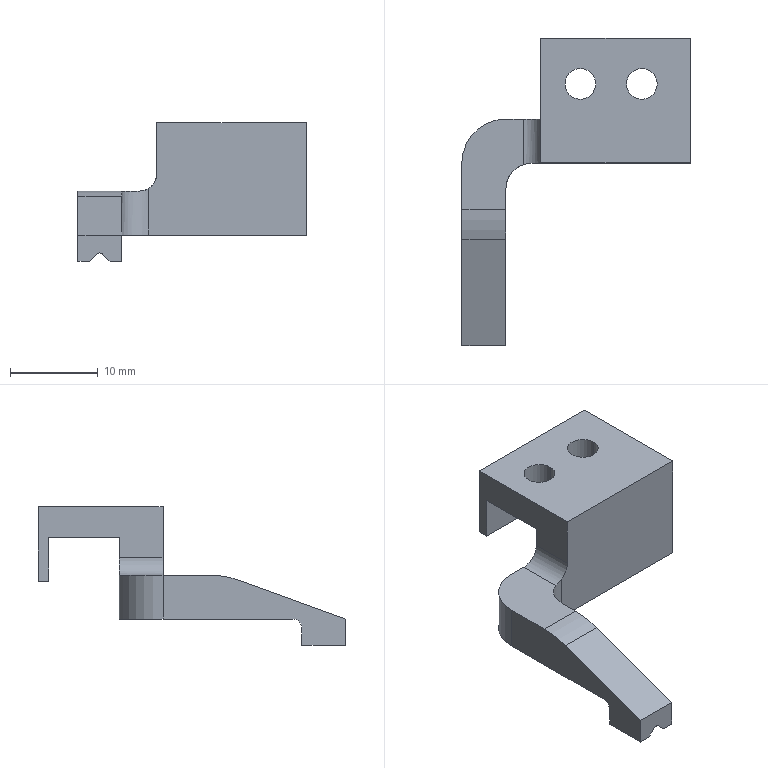Part | SolidWorks | features ICE 10, Fillet 6, Chamfer 1, Extrusion 1, HoleWzd 1, MoveFace 1 | 1 solid | 31 faces | box 26 x 35 x 15.8 mm | volume 2299 mm3 | plane 20 | cylinder 11 | commonest cylinder face diameters 3.5 x4 1 x2 2 x1 4 x1 6 x1 10 x1
STEP:
#1=CARTESIAN_POINT('',(-10.5,-18.5,-6.943));
#2=VERTEX_POINT('',#1);
#3=CARTESIAN_POINT('',(-10.146,-18.5,-7.089));
#4=VERTEX_POINT('',#3);
#5=CARTESIAN_POINT('',(-10.5,-18.5,-7.443));
#6=DIRECTION('',(0.,1.,0.));
#7=DIRECTION('',(0.,0.,1.));
#8=AXIS2_PLACEMENT_3D('',#5,#6,#7);
#9=CIRCLE('',#8,0.5);
#10=EDGE_CURVE('',#2,#4,#9,.T.);
#11=ORIENTED_EDGE('',*,*,#10,.F.);
#12=CARTESIAN_POINT('',(-10.5,-13.5,-6.943));
#13=VERTEX_POINT('',#12);
#14=CARTESIAN_POINT('',(-10.5,4.5,-6.943));
#15=DIRECTION('',(0.,1.,0.));
#16=VECTOR('',#15,1000.);
#17=LINE('',#14,#16);
#18=EDGE_CURVE('',#2,#13,#17,.T.);
#19=ORIENTED_EDGE('',*,*,#18,.T.);
#20=CARTESIAN_POINT('',(-10.146,-13.5,-7.089));
#21=VERTEX_POINT('',#20);
#22=CARTESIAN_POINT('',(-10.5,-13.5,-7.443));
#23=DIRECTION('',(0.,-1.,0.));
#24=DIRECTION('',(0.,0.,1.));
#25=AXIS2_PLACEMENT_3D('',#22,#23,#24);
#26=CIRCLE('',#25,0.5);
#27=EDGE_CURVE('',#21,#13,#26,.T.);
#28=ORIENTED_EDGE('',*,*,#27,.F.);
#29=CARTESIAN_POINT('',(-10.146,-11.5,-7.089));
#30=DIRECTION('',(0.,1.,0.));
#31=VECTOR('',#30,1000.);
#32=LINE('',#29,#31);
#33=EDGE_CURVE('',#4,#21,#32,.T.);
#34=ORIENTED_EDGE('',*,*,#33,.F.);
#35=EDGE_LOOP('',(#11,#19,#28,#34));
#36=FACE_OUTER_BOUND('',#35,.T.);
#37=CARTESIAN_POINT('',(-10.5,4.5,-7.443));
#38=DIRECTION('',(0.,1.,0.));
#39=DIRECTION('',(0.,0.,1.));
#40=AXIS2_PLACEMENT_3D('',#37,#38,#39);
#41=CYLINDRICAL_SURFACE('',#40,0.5);
#42=ADVANCED_FACE('',(#36),#41,.F.);
#43=CARTESIAN_POINT('',(2.25,11.3,4.4));
#44=VERTEX_POINT('',#43);
#45=CARTESIAN_POINT('',(-1.25,11.3,4.4));
#46=VERTEX_POINT('',#45);
#47=CARTESIAN_POINT('',(0.5,11.3,4.4));
#48=DIRECTION('',(0.,0.,-1.));
#49=DIRECTION('',(1.,0.,0.));
#50=AXIS2_PLACEMENT_3D('',#47,#48,#49);
#51=CIRCLE('',#50,1.75);
#52=EDGE_CURVE('',#44,#46,#51,.T.);
#53=ORIENTED_EDGE('',*,*,#52,.T.);
#54=CARTESIAN_POINT('',(-1.25,11.3,7.9));
#55=VERTEX_POINT('',#54);
#56=CARTESIAN_POINT('',(-1.25,11.3,7.9));
#57=DIRECTION('',(0.,0.,1.));
#58=VECTOR('',#57,1000.);
#59=LINE('',#56,#58);
#60=EDGE_CURVE('',#46,#55,#59,.T.);
#61=ORIENTED_EDGE('',*,*,#60,.T.);
#62=CARTESIAN_POINT('',(2.25,11.3,7.9));
#63=VERTEX_POINT('',#62);
#64=CARTESIAN_POINT('',(0.5,11.3,7.9));
#65=DIRECTION('',(0.,0.,1.));
#66=DIRECTION('',(1.,0.,0.));
#67=AXIS2_PLACEMENT_3D('',#64,#65,#66);
#68=CIRCLE('',#67,1.75);
#69=EDGE_CURVE('',#55,#63,#68,.T.);
#70=ORIENTED_EDGE('',*,*,#69,.T.);
#71=CARTESIAN_POINT('',(2.25,11.3,7.9));
#72=DIRECTION('',(0.,0.,1.));
#73=VECTOR('',#72,1000.);
#74=LINE('',#71,#73);
#75=EDGE_CURVE('',#44,#63,#74,.T.);
#76=ORIENTED_EDGE('',*,*,#75,.F.);
#77=EDGE_LOOP('',(#53,#61,#70,#76));
#78=FACE_OUTER_BOUND('',#77,.T.);
#79=CARTESIAN_POINT('',(0.5,11.3,7.9));
#80=DIRECTION('',(0.,0.,1.));
#81=DIRECTION('',(1.,0.,0.));
#82=AXIS2_PLACEMENT_3D('',#79,#80,#81);
#83=CYLINDRICAL_SURFACE('',#82,1.75);
#84=ADVANCED_FACE('',(#78),#83,.F.);
#85=CARTESIAN_POINT('',(9.25,11.3,4.4));
#86=VERTEX_POINT('',#85);
#87=CARTESIAN_POINT('',(5.75,11.3,4.4));
#88=VERTEX_POINT('',#87);
#89=CARTESIAN_POINT('',(7.5,11.3,4.4));
#90=DIRECTION('',(0.,0.,-1.));
#91=DIRECTION('',(1.,0.,0.));
#92=AXIS2_PLACEMENT_3D('',#89,#90,#91);
#93=CIRCLE('',#92,1.75);
#94=EDGE_CURVE('',#86,#88,#93,.T.);
#95=ORIENTED_EDGE('',*,*,#94,.T.);
#96=CARTESIAN_POINT('',(5.75,11.3,7.9));
#97=VERTEX_POINT('',#96);
#98=CARTESIAN_POINT('',(5.75,11.3,7.9));
#99=DIRECTION('',(0.,0.,1.));
#100=VECTOR('',#99,1000.);
#101=LINE('',#98,#100);
#102=EDGE_CURVE('',#88,#97,#101,.T.);
#103=ORIENTED_EDGE('',*,*,#102,.T.);
#104=CARTESIAN_POINT('',(9.25,11.3,7.9));
#105=VERTEX_POINT('',#104);
#106=CARTESIAN_POINT('',(7.5,11.3,7.9));
#107=DIRECTION('',(0.,0.,1.));
#108=DIRECTION('',(1.,0.,0.));
#109=AXIS2_PLACEMENT_3D('',#106,#107,#108);
#110=CIRCLE('',#109,1.75);
#111=EDGE_CURVE('',#97,#105,#110,.T.);
#112=ORIENTED_EDGE('',*,*,#111,.T.);
#113=CARTESIAN_POINT('',(9.25,11.3,7.9));
#114=DIRECTION('',(0.,0.,1.));
#115=VECTOR('',#114,1000.);
#116=LINE('',#113,#115);
#117=EDGE_CURVE('',#86,#105,#116,.T.);
#118=ORIENTED_EDGE('',*,*,#117,.F.);
#119=EDGE_LOOP('',(#95,#103,#112,#118));
#120=FACE_OUTER_BOUND('',#119,.T.);
#121=CARTESIAN_POINT('',(7.5,11.3,7.9));
#122=DIRECTION('',(0.,0.,1.));
#123=DIRECTION('',(1.,0.,0.));
#124=AXIS2_PLACEMENT_3D('',#121,#122,#123);
#125=CYLINDRICAL_SURFACE('',#124,1.75);
#126=ADVANCED_FACE('',(#120),#125,.F.);
#127=CARTESIAN_POINT('',(-9.336,-18.5,-7.9));
#128=VERTEX_POINT('',#127);
#129=CARTESIAN_POINT('',(-8.,-18.5,-7.9));
#130=VERTEX_POINT('',#129);
#131=CARTESIAN_POINT('',(-13.,-18.5,-7.9));
#132=DIRECTION('',(1.,0.,0.));
#133=VECTOR('',#132,1000.);
#134=LINE('',#131,#133);
#135=EDGE_CURVE('',#128,#130,#134,.T.);
#136=ORIENTED_EDGE('',*,*,#135,.F.);
#137=CARTESIAN_POINT('',(-9.336,-13.5,-7.9));
#138=VERTEX_POINT('',#137);
#139=CARTESIAN_POINT('',(-9.336,0.,-7.9));
#140=DIRECTION('',(0.,1.,0.));
#141=VECTOR('',#140,1000.);
#142=LINE('',#139,#141);
#143=EDGE_CURVE('',#128,#138,#142,.T.);
#144=ORIENTED_EDGE('',*,*,#143,.T.);
#145=CARTESIAN_POINT('',(-8.,-13.5,-7.9));
#146=VERTEX_POINT('',#145);
#147=CARTESIAN_POINT('',(-13.,-13.5,-7.9));
#148=DIRECTION('',(1.,0.,0.));
#149=VECTOR('',#148,1000.);
#150=LINE('',#147,#149);
#151=EDGE_CURVE('',#138,#146,#150,.T.);
#152=ORIENTED_EDGE('',*,*,#151,.T.);
#153=CARTESIAN_POINT('',(-8.,-16.5,-7.9));
#154=DIRECTION('',(0.,-1.,0.));
#155=VECTOR('',#154,1000.);
#156=LINE('',#153,#155);
#157=EDGE_CURVE('',#146,#130,#156,.T.);
#158=ORIENTED_EDGE('',*,*,#157,.T.);
#159=EDGE_LOOP('',(#136,#144,#152,#158));
#160=FACE_OUTER_BOUND('',#159,.T.);
#161=CARTESIAN_POINT('',(0.,0.,-7.9));
#162=DIRECTION('',(0.,0.,1.));
#163=DIRECTION('',(1.,0.,0.));
#164=AXIS2_PLACEMENT_3D('',#161,#162,#163);
#165=PLANE('',#164);
#166=ADVANCED_FACE('',(#160),#165,.F.);
#167=CARTESIAN_POINT('',(-13.,-6.42,-0.5031));
#168=VERTEX_POINT('',#167);
#169=CARTESIAN_POINT('',(-13.,-18.5,-4.9));
#170=VERTEX_POINT('',#169);
#171=CARTESIAN_POINT('',(-13.,-18.5,-4.9));
#172=DIRECTION('',(0.,-0.9397,-0.342));
#173=VECTOR('',#172,1000.);
#174=LINE('',#171,#173);
#175=EDGE_CURVE('',#168,#170,#174,.T.);
#176=ORIENTED_EDGE('',*,*,#175,.F.);
#177=CARTESIAN_POINT('',(-13.,-2.999,0.1));
#178=VERTEX_POINT('',#177);
#179=CARTESIAN_POINT('',(-13.,-2.999,-9.9));
#180=DIRECTION('',(-1.,0.,0.));
#181=DIRECTION('',(0.,1.,0.));
#182=AXIS2_PLACEMENT_3D('',#179,#180,#181);
#183=CIRCLE('',#182,10.);
#184=EDGE_CURVE('',#168,#178,#183,.T.);
#185=ORIENTED_EDGE('',*,*,#184,.T.);
#186=CARTESIAN_POINT('',(-13.,2.3,0.1));
#187=VERTEX_POINT('',#186);
#188=CARTESIAN_POINT('',(-13.,-16.5,0.1));
#189=DIRECTION('',(0.,-1.,0.));
#190=VECTOR('',#189,1000.);
#191=LINE('',#188,#190);
#192=EDGE_CURVE('',#187,#178,#191,.T.);
#193=ORIENTED_EDGE('',*,*,#192,.F.);
#194=CARTESIAN_POINT('',(-13.,2.3,-4.9));
#195=VERTEX_POINT('',#194);
#196=CARTESIAN_POINT('',(-13.,2.3,7.9));
#197=DIRECTION('',(0.,0.,-1.));
#198=VECTOR('',#197,1000.);
#199=LINE('',#196,#198);
#200=EDGE_CURVE('',#187,#195,#199,.T.);
#201=ORIENTED_EDGE('',*,*,#200,.T.);
#202=CARTESIAN_POINT('',(-13.,-12.5,-4.9));
#203=VERTEX_POINT('',#202);
#204=CARTESIAN_POINT('',(-13.,-25.044,-4.9));
#205=DIRECTION('',(0.,1.,0.));
#206=VECTOR('',#205,1000.);
#207=LINE('',#204,#206);
#208=EDGE_CURVE('',#203,#195,#207,.T.);
#209=ORIENTED_EDGE('',*,*,#208,.F.);
#210=CARTESIAN_POINT('',(-13.,-13.5,-5.9));
#211=VERTEX_POINT('',#210);
#212=CARTESIAN_POINT('',(-13.,-12.5,-5.9));
#213=DIRECTION('',(1.,0.,0.));
#214=DIRECTION('',(0.,1.,0.));
#215=AXIS2_PLACEMENT_3D('',#212,#213,#214);
#216=CIRCLE('',#215,1.);
#217=EDGE_CURVE('',#203,#211,#216,.T.);
#218=ORIENTED_EDGE('',*,*,#217,.T.);
#219=CARTESIAN_POINT('',(-13.,-13.5,-7.9));
#220=VERTEX_POINT('',#219);
#221=CARTESIAN_POINT('',(-13.,-13.5,-7.9));
#222=DIRECTION('',(0.,0.,-1.));
#223=VECTOR('',#222,1000.);
#224=LINE('',#221,#223);
#225=EDGE_CURVE('',#211,#220,#224,.T.);
#226=ORIENTED_EDGE('',*,*,#225,.T.);
#227=CARTESIAN_POINT('',(-13.,-18.5,-7.9));
#228=VERTEX_POINT('',#227);
#229=CARTESIAN_POINT('',(-13.,16.5,-7.9));
#230=DIRECTION('',(0.,-1.,0.));
#231=VECTOR('',#230,1000.);
#232=LINE('',#229,#231);
#233=EDGE_CURVE('',#220,#228,#232,.T.);
#234=ORIENTED_EDGE('',*,*,#233,.T.);
#235=CARTESIAN_POINT('',(-13.,-18.5,7.9));
#236=DIRECTION('',(0.,0.,-1.));
#237=VECTOR('',#236,1000.);
#238=LINE('',#235,#237);
#239=EDGE_CURVE('',#170,#228,#238,.T.);
#240=ORIENTED_EDGE('',*,*,#239,.F.);
#241=EDGE_LOOP('',(#176,#185,#193,#201,#209,#218,#226,#234,#240));
#242=FACE_OUTER_BOUND('',#241,.T.);
#243=CARTESIAN_POINT('',(-13.,16.5,7.9));
#244=DIRECTION('',(1.,0.,0.));
#245=DIRECTION('',(0.,1.,0.));
#246=AXIS2_PLACEMENT_3D('',#243,#244,#245);
#247=PLANE('',#246);
#248=ADVANCED_FACE('',(#242),#247,.F.);
#249=CARTESIAN_POINT('',(-10.854,-18.5,-7.089));
#250=VERTEX_POINT('',#249);
#251=CARTESIAN_POINT('',(-11.664,-18.5,-7.9));
#252=VERTEX_POINT('',#251);
#253=CARTESIAN_POINT('',(-10.5,-18.5,-6.736));
#254=DIRECTION('',(-0.7071,0.,-0.7071));
#255=VECTOR('',#254,1000.);
#256=LINE('',#253,#255);
#257=EDGE_CURVE('',#250,#252,#256,.T.);
#258=ORIENTED_EDGE('',*,*,#257,.F.);
#259=CARTESIAN_POINT('',(-10.5,-18.5,-7.443));
#260=DIRECTION('',(0.,1.,0.));
#261=DIRECTION('',(0.,0.,1.));
#262=AXIS2_PLACEMENT_3D('',#259,#260,#261);
#263=CIRCLE('',#262,0.5);
#264=EDGE_CURVE('',#250,#2,#263,.T.);
#265=ORIENTED_EDGE('',*,*,#264,.T.);
#266=ORIENTED_EDGE('',*,*,#10,.T.);
#267=CARTESIAN_POINT('',(-8.131,-18.5,-9.104));
#268=DIRECTION('',(-0.7071,0.,0.7071));
#269=VECTOR('',#268,1000.);
#270=LINE('',#267,#269);
#271=EDGE_CURVE('',#128,#4,#270,.T.);
#272=ORIENTED_EDGE('',*,*,#271,.F.);
#273=ORIENTED_EDGE('',*,*,#135,.T.);
#274=CARTESIAN_POINT('',(-8.,-18.5,-4.9));
#275=VERTEX_POINT('',#274);
#276=CARTESIAN_POINT('',(-8.,-18.5,-7.9));
#277=DIRECTION('',(0.,0.,1.));
#278=VECTOR('',#277,1000.);
#279=LINE('',#276,#278);
#280=EDGE_CURVE('',#130,#275,#279,.T.);
#281=ORIENTED_EDGE('',*,*,#280,.T.);
#282=CARTESIAN_POINT('',(-3.,-18.5,-4.9));
#283=DIRECTION('',(-1.,0.,0.));
#284=VECTOR('',#283,1000.);
#285=LINE('',#282,#284);
#286=EDGE_CURVE('',#275,#170,#285,.T.);
#287=ORIENTED_EDGE('',*,*,#286,.T.);
#288=ORIENTED_EDGE('',*,*,#239,.T.);
#289=CARTESIAN_POINT('',(-13.,-18.5,-7.9));
#290=DIRECTION('',(1.,0.,0.));
#291=VECTOR('',#290,1000.);
#292=LINE('',#289,#291);
#293=EDGE_CURVE('',#228,#252,#292,.T.);
#294=ORIENTED_EDGE('',*,*,#293,.T.);
#295=EDGE_LOOP('',(#258,#265,#266,#272,#273,#281,#287,#288,#294));
#296=FACE_OUTER_BOUND('',#295,.T.);
#297=CARTESIAN_POINT('',(-13.,-18.5,7.9));
#298=DIRECTION('',(0.,1.,0.));
#299=DIRECTION('',(0.,0.,1.));
#300=AXIS2_PLACEMENT_3D('',#297,#298,#299);
#301=PLANE('',#300);
#302=ADVANCED_FACE('',(#296),#301,.F.);
#303=CARTESIAN_POINT('',(0.5,11.3,7.9));
#304=DIRECTION('',(0.,0.,1.));
#305=DIRECTION('',(1.,0.,0.));
#306=AXIS2_PLACEMENT_3D('',#303,#304,#305);
#307=CIRCLE('',#306,1.75);
#308=EDGE_CURVE('',#63,#55,#307,.T.);
#309=ORIENTED_EDGE('',*,*,#308,.F.);
#310=ORIENTED_EDGE('',*,*,#69,.F.);
#311=EDGE_LOOP('',(#309,#310));
#312=FACE_BOUND('',#311,.T.);
#313=CARTESIAN_POINT('',(7.5,11.3,7.9));
#314=DIRECTION('',(0.,0.,1.));
#315=DIRECTION('',(1.,0.,0.));
#316=AXIS2_PLACEMENT_3D('',#313,#314,#315);
#317=CIRCLE('',#316,1.75);
#318=EDGE_CURVE('',#105,#97,#317,.T.);
#319=ORIENTED_EDGE('',*,*,#318,.F.);
#320=ORIENTED_EDGE('',*,*,#111,.F.);
#321=EDGE_LOOP('',(#319,#320));
#322=FACE_BOUND('',#321,.T.);
#323=CARTESIAN_POINT('',(-4.,16.5,7.9));
#324=VERTEX_POINT('',#323);
#325=CARTESIAN_POINT('',(-4.,2.3,7.9));
#326=VERTEX_POINT('',#325);
#327=CARTESIAN_POINT('',(-4.,7.3,7.9));
#328=DIRECTION('',(0.,-1.,0.));
#329=VECTOR('',#328,1000.);
#330=LINE('',#327,#329);
#331=EDGE_CURVE('',#324,#326,#330,.T.);
#332=ORIENTED_EDGE('',*,*,#331,.T.);
#333=CARTESIAN_POINT('',(13.,2.3,7.9));
#334=VERTEX_POINT('',#333);
#335=CARTESIAN_POINT('',(13.,2.3,7.9));
#336=DIRECTION('',(-1.,0.,0.));
#337=VECTOR('',#336,1000.);
#338=LINE('',#335,#337);
#339=EDGE_CURVE('',#334,#326,#338,.T.);
#340=ORIENTED_EDGE('',*,*,#339,.F.);
#341=CARTESIAN_POINT('',(13.,16.5,7.9));
#342=VERTEX_POINT('',#341);
#343=CARTESIAN_POINT('',(13.,16.5,7.9));
#344=DIRECTION('',(0.,1.,0.));
#345=VECTOR('',#344,1000.);
#346=LINE('',#343,#345);
#347=EDGE_CURVE('',#334,#342,#346,.T.);
#348=ORIENTED_EDGE('',*,*,#347,.T.);
#349=CARTESIAN_POINT('',(-13.,16.5,7.9));
#350=DIRECTION('',(-1.,0.,0.));
#351=VECTOR('',#350,1000.);
#352=LINE('',#349,#351);
#353=EDGE_CURVE('',#342,#324,#352,.T.);
#354=ORIENTED_EDGE('',*,*,#353,.T.);
#355=EDGE_LOOP('',(#332,#340,#348,#354));
#356=FACE_OUTER_BOUND('',#355,.T.);
#357=CARTESIAN_POINT('',(0.,0.,7.9));
#358=DIRECTION('',(0.,0.,1.));
#359=DIRECTION('',(1.,0.,0.));
#360=AXIS2_PLACEMENT_3D('',#357,#358,#359);
#361=PLANE('',#360);
#362=ADVANCED_FACE('',(#312,#322,#356),#361,.T.);
#363=CARTESIAN_POINT('',(-8.,7.3,-4.9));
#364=VERTEX_POINT('',#363);
#365=CARTESIAN_POINT('',(13.,7.3,-4.9));
#366=VERTEX_POINT('',#365);
#367=CARTESIAN_POINT('',(-5.,7.3,-4.9));
#368=DIRECTION('',(1.,0.,0.));
#369=VECTOR('',#368,1000.);
#370=LINE('',#367,#369);
#371=EDGE_CURVE('',#364,#366,#370,.T.);
#372=ORIENTED_EDGE('',*,*,#371,.F.);
#373=CARTESIAN_POINT('',(-8.,7.3,0.1));
#374=VERTEX_POINT('',#373);
#375=CARTESIAN_POINT('',(-8.,7.3,66.735));
#376=DIRECTION('',(0.,0.,1.));
#377=VECTOR('',#376,1000.);
#378=LINE('',#375,#377);
#379=EDGE_CURVE('',#364,#374,#378,.T.);
#380=ORIENTED_EDGE('',*,*,#379,.T.);
#381=CARTESIAN_POINT('',(-6.,7.3,0.1));
#382=VERTEX_POINT('',#381);
#383=CARTESIAN_POINT('',(-13.,7.3,0.1));
#384=DIRECTION('',(1.,0.,0.));
#385=VECTOR('',#384,1000.);
#386=LINE('',#383,#385);
#387=EDGE_CURVE('',#374,#382,#386,.T.);
#388=ORIENTED_EDGE('',*,*,#387,.T.);
#389=CARTESIAN_POINT('',(-4.,7.3,2.1));
#390=VERTEX_POINT('',#389);
#391=CARTESIAN_POINT('',(-6.,7.3,2.1));
#392=DIRECTION('',(0.,-1.,0.));
#393=DIRECTION('',(0.,0.,-1.));
#394=AXIS2_PLACEMENT_3D('',#391,#392,#393);
#395=CIRCLE('',#394,2.);
#396=EDGE_CURVE('',#382,#390,#395,.T.);
#397=ORIENTED_EDGE('',*,*,#396,.T.);
#398=CARTESIAN_POINT('',(-4.,7.3,4.4));
#399=VERTEX_POINT('',#398);
#400=CARTESIAN_POINT('',(-4.,7.3,7.9));
#401=DIRECTION('',(0.,0.,-1.));
#402=VECTOR('',#401,1000.);
#403=LINE('',#400,#402);
#404=EDGE_CURVE('',#399,#390,#403,.T.);
#405=ORIENTED_EDGE('',*,*,#404,.F.);
#406=CARTESIAN_POINT('',(13.,7.3,4.4));
#407=VERTEX_POINT('',#406);
#408=CARTESIAN_POINT('',(39.232,7.3,4.4));
#409=DIRECTION('',(-1.,0.,0.));
#410=VECTOR('',#409,1000.);
#411=LINE('',#408,#410);
#412=EDGE_CURVE('',#407,#399,#411,.T.);
#413=ORIENTED_EDGE('',*,*,#412,.F.);
#414=CARTESIAN_POINT('',(13.,7.3,7.9));
#415=DIRECTION('',(0.,0.,1.));
#416=VECTOR('',#415,1000.);
#417=LINE('',#414,#416);
#418=EDGE_CURVE('',#366,#407,#417,.T.);
#419=ORIENTED_EDGE('',*,*,#418,.F.);
#420=EDGE_LOOP('',(#372,#380,#388,#397,#405,#413,#419));
#421=FACE_OUTER_BOUND('',#420,.T.);
#422=CARTESIAN_POINT('',(39.232,7.3,66.735));
#423=DIRECTION('',(0.,-1.,0.));
#424=DIRECTION('',(0.,0.,-1.));
#425=AXIS2_PLACEMENT_3D('',#422,#423,#424);
#426=PLANE('',#425);
#427=ADVANCED_FACE('',(#421),#426,.F.);
#428=CARTESIAN_POINT('',(-4.,2.3,2.1));
#429=VERTEX_POINT('',#428);
#430=CARTESIAN_POINT('',(-4.,2.3,-7.9));
#431=DIRECTION('',(0.,0.,1.));
#432=VECTOR('',#431,1000.);
#433=LINE('',#430,#432);
#434=EDGE_CURVE('',#429,#326,#433,.T.);
#435=ORIENTED_EDGE('',*,*,#434,.F.);
#436=CARTESIAN_POINT('',(-5.,2.3,0.3679));
#437=VERTEX_POINT('',#436);
#438=CARTESIAN_POINT('',(-6.,2.3,2.1));
#439=DIRECTION('',(0.,1.,0.));
#440=DIRECTION('',(-1.,0.,0.));
#441=AXIS2_PLACEMENT_3D('',#438,#439,#440);
#442=CIRCLE('',#441,2.);
#443=EDGE_CURVE('',#429,#437,#442,.T.);
#444=ORIENTED_EDGE('',*,*,#443,.T.);
#445=CARTESIAN_POINT('',(-5.,2.3,-4.9));
#446=VERTEX_POINT('',#445);
#447=CARTESIAN_POINT('',(-5.,2.3,-4.9));
#448=DIRECTION('',(0.,0.,-1.));
#449=VECTOR('',#448,1000.);
#450=LINE('',#447,#449);
#451=EDGE_CURVE('',#437,#446,#450,.T.);
#452=ORIENTED_EDGE('',*,*,#451,.T.);
#453=CARTESIAN_POINT('',(13.,2.3,-4.9));
#454=VERTEX_POINT('',#453);
#455=CARTESIAN_POINT('',(-5.,2.3,-4.9));
#456=DIRECTION('',(-1.,0.,0.));
#457=VECTOR('',#456,1000.);
#458=LINE('',#455,#457);
#459=EDGE_CURVE('',#454,#446,#458,.T.);
#460=ORIENTED_EDGE('',*,*,#459,.F.);
#461=CARTESIAN_POINT('',(13.,2.3,-7.9));
#462=DIRECTION('',(0.,0.,1.));
#463=VECTOR('',#462,1000.);
#464=LINE('',#461,#463);
#465=EDGE_CURVE('',#454,#334,#464,.T.);
#466=ORIENTED_EDGE('',*,*,#465,.T.);
#467=ORIENTED_EDGE('',*,*,#339,.T.);
#468=EDGE_LOOP('',(#435,#444,#452,#460,#466,#467));
#469=FACE_OUTER_BOUND('',#468,.T.);
#470=CARTESIAN_POINT('',(13.,2.3,-7.9));
#471=DIRECTION('',(0.,1.,0.));
#472=DIRECTION('',(-1.,0.,0.));
#473=AXIS2_PLACEMENT_3D('',#470,#471,#472);
#474=PLANE('',#473);
#475=ADVANCED_FACE('',(#469),#474,.F.);
#476=CARTESIAN_POINT('',(-8.,-2.999,0.1));
#477=VERTEX_POINT('',#476);
#478=CARTESIAN_POINT('',(-8.,-0.7,0.1));
#479=VERTEX_POINT('',#478);
#480=CARTESIAN_POINT('',(-8.,-16.5,0.1));
#481=DIRECTION('',(0.,1.,0.));
#482=VECTOR('',#481,1000.);
#483=LINE('',#480,#482);
#484=EDGE_CURVE('',#477,#479,#483,.T.);
#485=ORIENTED_EDGE('',*,*,#484,.F.);
#486=CARTESIAN_POINT('',(-8.,-6.42,-0.5031));
#487=VERTEX_POINT('',#486);
#488=CARTESIAN_POINT('',(-8.,-2.999,-9.9));
#489=DIRECTION('',(1.,0.,0.));
#490=DIRECTION('',(0.,0.,1.));
#491=AXIS2_PLACEMENT_3D('',#488,#489,#490);
#492=CIRCLE('',#491,10.);
#493=EDGE_CURVE('',#477,#487,#492,.T.);
#494=ORIENTED_EDGE('',*,*,#493,.T.);
#495=CARTESIAN_POINT('',(-8.,-19.464,-5.251));
#496=DIRECTION('',(0.,-0.9397,-0.342));
#497=VECTOR('',#496,1000.);
#498=LINE('',#495,#497);
#499=EDGE_CURVE('',#487,#275,#498,.T.);
#500=ORIENTED_EDGE('',*,*,#499,.T.);
#501=ORIENTED_EDGE('',*,*,#280,.F.);
#502=ORIENTED_EDGE('',*,*,#157,.F.);
#503=CARTESIAN_POINT('',(-8.,-13.5,-5.9));
#504=VERTEX_POINT('',#503);
#505=CARTESIAN_POINT('',(-8.,-13.5,7.9));
#506=DIRECTION('',(0.,0.,1.));
#507=VECTOR('',#506,1000.);
#508=LINE('',#505,#507);
#509=EDGE_CURVE('',#146,#504,#508,.T.);
#510=ORIENTED_EDGE('',*,*,#509,.T.);
#511=CARTESIAN_POINT('',(-8.,-12.5,-4.9));
#512=VERTEX_POINT('',#511);
#513=CARTESIAN_POINT('',(-8.,-12.5,-5.9));
#514=DIRECTION('',(-1.,0.,0.));
#515=DIRECTION('',(0.,0.,1.));
#516=AXIS2_PLACEMENT_3D('',#513,#514,#515);
#517=CIRCLE('',#516,1.);
#518=EDGE_CURVE('',#504,#512,#517,.T.);
#519=ORIENTED_EDGE('',*,*,#518,.T.);
#520=CARTESIAN_POINT('',(-8.,-0.7,-4.9));
#521=VERTEX_POINT('',#520);
#522=CARTESIAN_POINT('',(-8.,-16.5,-4.9));
#523=DIRECTION('',(0.,-1.,0.));
#524=VECTOR('',#523,1000.);
#525=LINE('',#522,#524);
#526=EDGE_CURVE('',#521,#512,#525,.T.);
#527=ORIENTED_EDGE('',*,*,#526,.F.);
#528=CARTESIAN_POINT('',(-8.,-0.7,0.1));
#529=DIRECTION('',(0.,0.,1.));
#530=VECTOR('',#529,1000.);
#531=LINE('',#528,#530);
#532=EDGE_CURVE('',#521,#479,#531,.T.);
#533=ORIENTED_EDGE('',*,*,#532,.T.);
#534=EDGE_LOOP('',(#485,#494,#500,#501,#502,#510,#519,#527,#533));
#535=FACE_OUTER_BOUND('',#534,.T.);
#536=CARTESIAN_POINT('',(-8.,-16.5,-7.9));
#537=DIRECTION('',(-1.,0.,0.));
#538=DIRECTION('',(0.,0.,1.));
#539=AXIS2_PLACEMENT_3D('',#536,#537,#538);
#540=PLANE('',#539);
#541=ADVANCED_FACE('',(#535),#540,.F.);
#542=CARTESIAN_POINT('',(-11.664,-13.5,-7.9));
#543=VERTEX_POINT('',#542);
#544=CARTESIAN_POINT('',(-13.,-13.5,-7.9));
#545=DIRECTION('',(1.,0.,0.));
#546=VECTOR('',#545,1000.);
#547=LINE('',#544,#546);
#548=EDGE_CURVE('',#220,#543,#547,.T.);
#549=ORIENTED_EDGE('',*,*,#548,.T.);
#550=CARTESIAN_POINT('',(-11.664,0.,-7.9));
#551=DIRECTION('',(0.,-1.,0.));
#552=VECTOR('',#551,1000.);
#553=LINE('',#550,#552);
#554=EDGE_CURVE('',#543,#252,#553,.T.);
#555=ORIENTED_EDGE('',*,*,#554,.T.);
#556=ORIENTED_EDGE('',*,*,#293,.F.);
#557=ORIENTED_EDGE('',*,*,#233,.F.);
#558=EDGE_LOOP('',(#549,#555,#556,#557));
#559=FACE_OUTER_BOUND('',#558,.T.);
#560=CARTESIAN_POINT('',(0.,0.,-7.9));
#561=DIRECTION('',(0.,0.,1.));
#562=DIRECTION('',(1.,0.,0.));
#563=AXIS2_PLACEMENT_3D('',#560,#561,#562);
#564=PLANE('',#563);
#565=ADVANCED_FACE('',(#559),#564,.F.);
#566=ORIENTED_EDGE('',*,*,#347,.F.);
#567=ORIENTED_EDGE('',*,*,#465,.F.);
#568=CARTESIAN_POINT('',(13.,-16.5,-4.9));
#569=DIRECTION('',(0.,1.,0.));
#570=VECTOR('',#569,1000.);
#571=LINE('',#568,#570);
#572=EDGE_CURVE('',#454,#366,#571,.T.);
#573=ORIENTED_EDGE('',*,*,#572,.T.);
#574=ORIENTED_EDGE('',*,*,#418,.T.);
#575=CARTESIAN_POINT('',(13.,15.3,4.4));
#576=VERTEX_POINT('',#575);
#577=CARTESIAN_POINT('',(13.,16.5,4.4));
#578=DIRECTION('',(0.,1.,0.));
#579=VECTOR('',#578,1000.);
#580=LINE('',#577,#579);
#581=EDGE_CURVE('',#407,#576,#580,.T.);
#582=ORIENTED_EDGE('',*,*,#581,.T.);
#583=CARTESIAN_POINT('',(13.,15.3,-0.6));
#584=VERTEX_POINT('',#583);
#585=CARTESIAN_POINT('',(13.,15.3,7.9));
#586=DIRECTION('',(0.,0.,-1.));
#587=VECTOR('',#586,1000.);
#588=LINE('',#585,#587);
#589=EDGE_CURVE('',#576,#584,#588,.T.);
#590=ORIENTED_EDGE('',*,*,#589,.T.);
#591=CARTESIAN_POINT('',(13.,16.5,-0.6));
#592=VERTEX_POINT('',#591);
#593=CARTESIAN_POINT('',(13.,16.5,-0.6));
#594=DIRECTION('',(0.,1.,0.));
#595=VECTOR('',#594,1000.);
#596=LINE('',#593,#595);
#597=EDGE_CURVE('',#584,#592,#596,.T.);
#598=ORIENTED_EDGE('',*,*,#597,.T.);
#599=CARTESIAN_POINT('',(13.,16.5,7.9));
#600=DIRECTION('',(0.,0.,-1.));
#601=VECTOR('',#600,1000.);
#602=LINE('',#599,#601);
#603=EDGE_CURVE('',#342,#592,#602,.T.);
#604=ORIENTED_EDGE('',*,*,#603,.F.);
#605=EDGE_LOOP('',(#566,#567,#573,#574,#582,#590,#598,#604));
#606=FACE_OUTER_BOUND('',#605,.T.);
#607=CARTESIAN_POINT('',(13.,16.5,7.9));
#608=DIRECTION('',(-1.,0.,0.));
#609=DIRECTION('',(0.,-1.,0.));
#610=AXIS2_PLACEMENT_3D('',#607,#608,#609);
#611=PLANE('',#610);
#612=ADVANCED_FACE('',(#606),#611,.F.);
#613=CARTESIAN_POINT('',(-4.,16.5,-0.6));
#614=VERTEX_POINT('',#613);
#615=CARTESIAN_POINT('',(13.,16.5,-0.6));
#616=DIRECTION('',(-1.,0.,0.));
#617=VECTOR('',#616,1000.);
#618=LINE('',#615,#617);
#619=EDGE_CURVE('',#592,#614,#618,.T.);
#620=ORIENTED_EDGE('',*,*,#619,.T.);
#621=CARTESIAN_POINT('',(-4.,16.5,7.9));
#622=DIRECTION('',(0.,0.,-1.));
#623=VECTOR('',#622,1000.);
#624=LINE('',#621,#623);
#625=EDGE_CURVE('',#324,#614,#624,.T.);
#626=ORIENTED_EDGE('',*,*,#625,.F.);
#627=ORIENTED_EDGE('',*,*,#353,.F.);
#628=ORIENTED_EDGE('',*,*,#603,.T.);
#629=EDGE_LOOP('',(#620,#626,#627,#628));
#630=FACE_OUTER_BOUND('',#629,.T.);
#631=CARTESIAN_POINT('',(-13.,16.5,7.9));
#632=DIRECTION('',(0.,-1.,0.));
#633=DIRECTION('',(0.,0.,-1.));
#634=AXIS2_PLACEMENT_3D('',#631,#632,#633);
#635=PLANE('',#634);
#636=ADVANCED_FACE('',(#630),#635,.F.);
#637=ORIENTED_EDGE('',*,*,#102,.F.);
#638=CARTESIAN_POINT('',(7.5,11.3,4.4));
#639=DIRECTION('',(0.,0.,-1.));
#640=DIRECTION('',(1.,0.,0.));
#641=AXIS2_PLACEMENT_3D('',#638,#639,#640);
#642=CIRCLE('',#641,1.75);
#643=EDGE_CURVE('',#88,#86,#642,.T.);
#644=ORIENTED_EDGE('',*,*,#643,.T.);
#645=ORIENTED_EDGE('',*,*,#117,.T.);
#646=ORIENTED_EDGE('',*,*,#318,.T.);
#647=EDGE_LOOP('',(#637,#644,#645,#646));
#648=FACE_OUTER_BOUND('',#647,.T.);
#649=CARTESIAN_POINT('',(7.5,11.3,7.9));
#650=DIRECTION('',(0.,0.,1.));
#651=DIRECTION('',(1.,0.,0.));
#652=AXIS2_PLACEMENT_3D('',#649,#650,#651);
#653=CYLINDRICAL_SURFACE('',#652,1.75);
#654=ADVANCED_FACE('',(#648),#653,.F.);
#655=ORIENTED_EDGE('',*,*,#60,.F.);
#656=CARTESIAN_POINT('',(0.5,11.3,4.4));
#657=DIRECTION('',(0.,0.,-1.));
#658=DIRECTION('',(1.,0.,0.));
#659=AXIS2_PLACEMENT_3D('',#656,#657,#658);
#660=CIRCLE('',#659,1.75);
#661=EDGE_CURVE('',#46,#44,#660,.T.);
#662=ORIENTED_EDGE('',*,*,#661,.T.);
#663=ORIENTED_EDGE('',*,*,#75,.T.);
#664=ORIENTED_EDGE('',*,*,#308,.T.);
#665=EDGE_LOOP('',(#655,#662,#663,#664));
#666=FACE_OUTER_BOUND('',#665,.T.);
#667=CARTESIAN_POINT('',(0.5,11.3,7.9));
#668=DIRECTION('',(0.,0.,1.));
#669=DIRECTION('',(1.,0.,0.));
#670=AXIS2_PLACEMENT_3D('',#667,#668,#669);
#671=CYLINDRICAL_SURFACE('',#670,1.75);
#672=ADVANCED_FACE('',(#666),#671,.F.);
#673=CARTESIAN_POINT('',(-4.,15.3,4.4));
#674=VERTEX_POINT('',#673);
#675=CARTESIAN_POINT('',(39.232,15.3,4.4));
#676=DIRECTION('',(1.,0.,0.));
#677=VECTOR('',#676,1000.);
#678=LINE('',#675,#677);
#679=EDGE_CURVE('',#674,#576,#678,.T.);
#680=ORIENTED_EDGE('',*,*,#679,.F.);
#681=CARTESIAN_POINT('',(-4.,15.3,-0.6));
#682=VERTEX_POINT('',#681);
#683=CARTESIAN_POINT('',(-4.,15.3,66.735));
#684=DIRECTION('',(0.,0.,-1.));
#685=VECTOR('',#684,1000.);
#686=LINE('',#683,#685);
#687=EDGE_CURVE('',#674,#682,#686,.T.);
#688=ORIENTED_EDGE('',*,*,#687,.T.);
#689=CARTESIAN_POINT('',(13.,15.3,-0.6));
#690=DIRECTION('',(-1.,0.,0.));
#691=VECTOR('',#690,1000.);
#692=LINE('',#689,#691);
#693=EDGE_CURVE('',#584,#682,#692,.T.);
#694=ORIENTED_EDGE('',*,*,#693,.F.);
#695=ORIENTED_EDGE('',*,*,#589,.F.);
#696=EDGE_LOOP('',(#680,#688,#694,#695));
#697=FACE_OUTER_BOUND('',#696,.T.);
#698=CARTESIAN_POINT('',(39.232,15.3,66.735));
#699=DIRECTION('',(0.,1.,0.));
#700=DIRECTION('',(0.,0.,1.));
#701=AXIS2_PLACEMENT_3D('',#698,#699,#700);
#702=PLANE('',#701);
#703=ADVANCED_FACE('',(#697),#702,.F.);
#704=ORIENTED_EDGE('',*,*,#52,.F.);
#705=ORIENTED_EDGE('',*,*,#661,.F.);
#706=EDGE_LOOP('',(#704,#705));
#707=FACE_BOUND('',#706,.T.);
#708=ORIENTED_EDGE('',*,*,#94,.F.);
#709=ORIENTED_EDGE('',*,*,#643,.F.);
#710=EDGE_LOOP('',(#708,#709));
#711=FACE_BOUND('',#710,.T.);
#712=ORIENTED_EDGE('',*,*,#412,.T.);
#713=CARTESIAN_POINT('',(-4.,0.,4.4));
#714=DIRECTION('',(0.,1.,0.));
#715=VECTOR('',#714,1000.);
#716=LINE('',#713,#715);
#717=EDGE_CURVE('',#399,#674,#716,.T.);
#718=ORIENTED_EDGE('',*,*,#717,.T.);
#719=ORIENTED_EDGE('',*,*,#679,.T.);
#720=ORIENTED_EDGE('',*,*,#581,.F.);
#721=EDGE_LOOP('',(#712,#718,#719,#720));
#722=FACE_OUTER_BOUND('',#721,.T.);
#723=CARTESIAN_POINT('',(0.,0.,4.4));
#724=DIRECTION('',(0.,0.,1.));
#725=DIRECTION('',(1.,0.,0.));
#726=AXIS2_PLACEMENT_3D('',#723,#724,#725);
#727=PLANE('',#726);
#728=ADVANCED_FACE('',(#707,#711,#722),#727,.F.);
#729=ORIENTED_EDGE('',*,*,#693,.T.);
#730=CARTESIAN_POINT('',(-4.,7.3,-0.6));
#731=DIRECTION('',(0.,-1.,0.));
#732=VECTOR('',#731,1000.);
#733=LINE('',#730,#732);
#734=EDGE_CURVE('',#614,#682,#733,.T.);
#735=ORIENTED_EDGE('',*,*,#734,.F.);
#736=ORIENTED_EDGE('',*,*,#619,.F.);
#737=ORIENTED_EDGE('',*,*,#597,.F.);
#738=EDGE_LOOP('',(#729,#735,#736,#737));
#739=FACE_OUTER_BOUND('',#738,.T.);
#740=CARTESIAN_POINT('',(13.,16.5,-0.6));
#741=DIRECTION('',(0.,0.,1.));
#742=DIRECTION('',(1.,0.,0.));
#743=AXIS2_PLACEMENT_3D('',#740,#741,#742);
#744=PLANE('',#743);
#745=ADVANCED_FACE('',(#739),#744,.F.);
#746=ORIENTED_EDGE('',*,*,#526,.T.);
#747=CARTESIAN_POINT('',(-5.,-12.5,-4.9));
#748=DIRECTION('',(-1.,0.,0.));
#749=VECTOR('',#748,1000.);
#750=LINE('',#747,#749);
#751=EDGE_CURVE('',#512,#203,#750,.T.);
#752=ORIENTED_EDGE('',*,*,#751,.T.);
#753=ORIENTED_EDGE('',*,*,#208,.T.);
#754=CARTESIAN_POINT('',(-8.,2.3,-4.9));
#755=DIRECTION('',(0.,0.,-1.));
#756=DIRECTION('',(1.,0.,0.));
#757=AXIS2_PLACEMENT_3D('',#754,#755,#756);
#758=CIRCLE('',#757,5.);
#759=EDGE_CURVE('',#195,#364,#758,.T.);
#760=ORIENTED_EDGE('',*,*,#759,.T.);
#761=ORIENTED_EDGE('',*,*,#371,.T.);
#762=ORIENTED_EDGE('',*,*,#572,.F.);
#763=ORIENTED_EDGE('',*,*,#459,.T.);
#764=CARTESIAN_POINT('',(-5.,-0.7,-4.9));
#765=DIRECTION('',(0.,0.,1.));
#766=DIRECTION('',(1.,0.,0.));
#767=AXIS2_PLACEMENT_3D('',#764,#765,#766);
#768=CIRCLE('',#767,3.);
#769=EDGE_CURVE('',#446,#521,#768,.T.);
#770=ORIENTED_EDGE('',*,*,#769,.T.);
#771=EDGE_LOOP('',(#746,#752,#753,#760,#761,#762,#763,#770));
#772=FACE_OUTER_BOUND('',#771,.T.);
#773=CARTESIAN_POINT('',(-5.,-16.5,-4.9));
#774=DIRECTION('',(0.,0.,1.));
#775=DIRECTION('',(1.,0.,0.));
#776=AXIS2_PLACEMENT_3D('',#773,#774,#775);
#777=PLANE('',#776);
#778=ADVANCED_FACE('',(#772),#777,.F.);
#779=ORIENTED_EDGE('',*,*,#225,.F.);
#780=CARTESIAN_POINT('',(-13.,-13.5,-5.9));
#781=DIRECTION('',(1.,0.,0.));
#782=VECTOR('',#781,1000.);
#783=LINE('',#780,#782);
#784=EDGE_CURVE('',#211,#504,#783,.T.);
#785=ORIENTED_EDGE('',*,*,#784,.T.);
#786=ORIENTED_EDGE('',*,*,#509,.F.);
#787=ORIENTED_EDGE('',*,*,#151,.F.);
#788=CARTESIAN_POINT('',(-19.068,-13.5,1.832));
#789=DIRECTION('',(0.7071,0.,-0.7071));
#790=VECTOR('',#789,1000.);
#791=LINE('',#788,#790);
#792=EDGE_CURVE('',#21,#138,#791,.T.);
#793=ORIENTED_EDGE('',*,*,#792,.F.);
#794=ORIENTED_EDGE('',*,*,#27,.T.);
#795=CARTESIAN_POINT('',(-10.854,-13.5,-7.089));
#796=VERTEX_POINT('',#795);
#797=CARTESIAN_POINT('',(-10.5,-13.5,-7.443));
#798=DIRECTION('',(0.,-1.,0.));
#799=DIRECTION('',(0.,0.,1.));
#800=AXIS2_PLACEMENT_3D('',#797,#798,#799);
#801=CIRCLE('',#800,0.5);
#802=EDGE_CURVE('',#13,#796,#801,.T.);
#803=ORIENTED_EDGE('',*,*,#802,.T.);
#804=CARTESIAN_POINT('',(-4.432,-13.5,-0.6679));
#805=DIRECTION('',(0.7071,0.,0.7071));
#806=VECTOR('',#805,1000.);
#807=LINE('',#804,#806);
#808=EDGE_CURVE('',#543,#796,#807,.T.);
#809=ORIENTED_EDGE('',*,*,#808,.F.);
#810=ORIENTED_EDGE('',*,*,#548,.F.);
#811=EDGE_LOOP('',(#779,#785,#786,#787,#793,#794,#803,#809,#810));
#812=FACE_OUTER_BOUND('',#811,.T.);
#813=CARTESIAN_POINT('',(-13.,-13.5,7.9));
#814=DIRECTION('',(0.,1.,0.));
#815=DIRECTION('',(0.,0.,1.));
#816=AXIS2_PLACEMENT_3D('',#813,#814,#815);
#817=PLANE('',#816);
#818=ADVANCED_FACE('',(#812),#817,.T.);
#819=ORIENTED_EDGE('',*,*,#404,.T.);
#820=CARTESIAN_POINT('',(-4.,7.3,2.1));
#821=DIRECTION('',(0.,-1.,0.));
#822=VECTOR('',#821,1000.);
#823=LINE('',#820,#822);
#824=EDGE_CURVE('',#390,#429,#823,.T.);
#825=ORIENTED_EDGE('',*,*,#824,.T.);
#826=ORIENTED_EDGE('',*,*,#434,.T.);
#827=ORIENTED_EDGE('',*,*,#331,.F.);
#828=ORIENTED_EDGE('',*,*,#625,.T.);
#829=ORIENTED_EDGE('',*,*,#734,.T.);
#830=ORIENTED_EDGE('',*,*,#687,.F.);
#831=ORIENTED_EDGE('',*,*,#717,.F.);
#832=EDGE_LOOP('',(#819,#825,#826,#827,#828,#829,#830,#831));
#833=FACE_OUTER_BOUND('',#832,.T.);
#834=CARTESIAN_POINT('',(-4.,7.3,7.9));
#835=DIRECTION('',(1.,0.,0.));
#836=DIRECTION('',(0.,0.,-1.));
#837=AXIS2_PLACEMENT_3D('',#834,#835,#836);
#838=PLANE('',#837);
#839=ADVANCED_FACE('',(#833),#838,.F.);
#840=ORIENTED_EDGE('',*,*,#192,.T.);
#841=CARTESIAN_POINT('',(-8.,-2.999,0.1));
#842=DIRECTION('',(1.,0.,0.));
#843=VECTOR('',#842,1000.);
#844=LINE('',#841,#843);
#845=EDGE_CURVE('',#178,#477,#844,.T.);
#846=ORIENTED_EDGE('',*,*,#845,.T.);
#847=ORIENTED_EDGE('',*,*,#484,.T.);
#848=CARTESIAN_POINT('',(-6.,2.128,0.1));
#849=VERTEX_POINT('',#848);
#850=CARTESIAN_POINT('',(-5.,-0.7,0.1));
#851=DIRECTION('',(0.,0.,-1.));
#852=DIRECTION('',(1.,0.,0.));
#853=AXIS2_PLACEMENT_3D('',#850,#851,#852);
#854=CIRCLE('',#853,3.);
#855=EDGE_CURVE('',#479,#849,#854,.T.);
#856=ORIENTED_EDGE('',*,*,#855,.T.);
#857=CARTESIAN_POINT('',(-6.,-16.5,0.1));
#858=DIRECTION('',(0.,1.,0.));
#859=VECTOR('',#858,1000.);
#860=LINE('',#857,#859);
#861=EDGE_CURVE('',#849,#382,#860,.T.);
#862=ORIENTED_EDGE('',*,*,#861,.T.);
#863=ORIENTED_EDGE('',*,*,#387,.F.);
#864=CARTESIAN_POINT('',(-8.,2.3,0.1));
#865=DIRECTION('',(0.,0.,1.));
#866=DIRECTION('',(1.,0.,0.));
#867=AXIS2_PLACEMENT_3D('',#864,#865,#866);
#868=CIRCLE('',#867,5.);
#869=EDGE_CURVE('',#374,#187,#868,.T.);
#870=ORIENTED_EDGE('',*,*,#869,.T.);
#871=EDGE_LOOP('',(#840,#846,#847,#856,#862,#863,#870));
#872=FACE_OUTER_BOUND('',#871,.T.);
#873=CARTESIAN_POINT('',(-13.,-16.5,0.1));
#874=DIRECTION('',(0.,0.,1.));
#875=DIRECTION('',(1.,0.,0.));
#876=AXIS2_PLACEMENT_3D('',#873,#874,#875);
#877=PLANE('',#876);
#878=ADVANCED_FACE('',(#872),#877,.T.);
#879=ORIENTED_EDGE('',*,*,#869,.F.);
#880=ORIENTED_EDGE('',*,*,#379,.F.);
#881=ORIENTED_EDGE('',*,*,#759,.F.);
#882=ORIENTED_EDGE('',*,*,#200,.F.);
#883=EDGE_LOOP('',(#879,#880,#881,#882));
#884=FACE_OUTER_BOUND('',#883,.T.);
#885=CARTESIAN_POINT('',(-8.,2.3,7.9));
#886=DIRECTION('',(0.,0.,-1.));
#887=DIRECTION('',(-1.,0.,0.));
#888=AXIS2_PLACEMENT_3D('',#885,#886,#887);
#889=CYLINDRICAL_SURFACE('',#888,5.);
#890=ADVANCED_FACE('',(#884),#889,.T.);
#891=ORIENTED_EDGE('',*,*,#769,.F.);
#892=ORIENTED_EDGE('',*,*,#451,.F.);
#893=CARTESIAN_POINT('',(-5.,2.3,0.3679));
#894=CARTESIAN_POINT('',(-5.155,2.3,0.2784));
#895=CARTESIAN_POINT('',(-5.318,2.288,0.2115));
#896=CARTESIAN_POINT('',(-5.659,2.232,0.1214));
#897=CARTESIAN_POINT('',(-5.831,2.188,0.1));
#898=CARTESIAN_POINT('',(-6.,2.128,0.1));
#899=B_SPLINE_CURVE_WITH_KNOTS('',3,(#893,#894,#895,#896,#897,#898),.UNSPECIFIED.,.F.,.F.,(4,2,4),(0.,0.0005299,0.00106),.UNSPECIFIED.);
#900=EDGE_CURVE('',#437,#849,#899,.T.);
#901=ORIENTED_EDGE('',*,*,#900,.T.);
#902=ORIENTED_EDGE('',*,*,#855,.F.);
#903=ORIENTED_EDGE('',*,*,#532,.F.);
#904=EDGE_LOOP('',(#891,#892,#901,#902,#903));
#905=FACE_OUTER_BOUND('',#904,.T.);
#906=CARTESIAN_POINT('',(-5.,-0.7,-7.9));
#907=DIRECTION('',(0.,0.,-1.));
#908=DIRECTION('',(-1.,0.,0.));
#909=AXIS2_PLACEMENT_3D('',#906,#907,#908);
#910=CYLINDRICAL_SURFACE('',#909,3.);
#911=ADVANCED_FACE('',(#905),#910,.F.);
#912=ORIENTED_EDGE('',*,*,#396,.F.);
#913=ORIENTED_EDGE('',*,*,#861,.F.);
#914=ORIENTED_EDGE('',*,*,#900,.F.);
#915=ORIENTED_EDGE('',*,*,#443,.F.);
#916=ORIENTED_EDGE('',*,*,#824,.F.);
#917=EDGE_LOOP('',(#912,#913,#914,#915,#916));
#918=FACE_OUTER_BOUND('',#917,.T.);
#919=CARTESIAN_POINT('',(-6.,7.3,2.1));
#920=DIRECTION('',(0.,-1.,0.));
#921=DIRECTION('',(0.,0.,-1.));
#922=AXIS2_PLACEMENT_3D('',#919,#920,#921);
#923=CYLINDRICAL_SURFACE('',#922,2.);
#924=ADVANCED_FACE('',(#918),#923,.F.);
#925=ORIENTED_EDGE('',*,*,#499,.F.);
#926=CARTESIAN_POINT('',(-13.,-6.42,-0.5031));
#927=DIRECTION('',(-1.,0.,0.));
#928=VECTOR('',#927,1000.);
#929=LINE('',#926,#928);
#930=EDGE_CURVE('',#487,#168,#929,.T.);
#931=ORIENTED_EDGE('',*,*,#930,.T.);
#932=ORIENTED_EDGE('',*,*,#175,.T.);
#933=ORIENTED_EDGE('',*,*,#286,.F.);
#934=EDGE_LOOP('',(#925,#931,#932,#933));
#935=FACE_OUTER_BOUND('',#934,.T.);
#936=CARTESIAN_POINT('',(-3.,-18.5,-4.9));
#937=DIRECTION('',(0.,0.342,-0.9397));
#938=DIRECTION('',(0.,0.9397,0.342));
#939=AXIS2_PLACEMENT_3D('',#936,#937,#938);
#940=PLANE('',#939);
#941=ADVANCED_FACE('',(#935),#940,.F.);
#942=ORIENTED_EDGE('',*,*,#271,.T.);
#943=ORIENTED_EDGE('',*,*,#33,.T.);
#944=ORIENTED_EDGE('',*,*,#792,.T.);
#945=ORIENTED_EDGE('',*,*,#143,.F.);
#946=EDGE_LOOP('',(#942,#943,#944,#945));
#947=FACE_OUTER_BOUND('',#946,.T.);
#948=CARTESIAN_POINT('',(-8.131,4.5,-9.104));
#949=DIRECTION('',(0.7071,0.,0.7071));
#950=DIRECTION('',(0.7071,0.,-0.7071));
#951=AXIS2_PLACEMENT_3D('',#948,#949,#950);
#952=PLANE('',#951);
#953=ADVANCED_FACE('',(#947),#952,.F.);
#954=ORIENTED_EDGE('',*,*,#808,.T.);
#955=CARTESIAN_POINT('',(-10.854,-16.5,-7.089));
#956=DIRECTION('',(0.,-1.,0.));
#957=VECTOR('',#956,1000.);
#958=LINE('',#955,#957);
#959=EDGE_CURVE('',#796,#250,#958,.T.);
#960=ORIENTED_EDGE('',*,*,#959,.T.);
#961=ORIENTED_EDGE('',*,*,#257,.T.);
#962=ORIENTED_EDGE('',*,*,#554,.F.);
#963=EDGE_LOOP('',(#954,#960,#961,#962));
#964=FACE_OUTER_BOUND('',#963,.T.);
#965=CARTESIAN_POINT('',(-10.5,4.5,-6.736));
#966=DIRECTION('',(-0.7071,0.,0.7071));
#967=DIRECTION('',(0.7071,0.,0.7071));
#968=AXIS2_PLACEMENT_3D('',#965,#966,#967);
#969=PLANE('',#968);
#970=ADVANCED_FACE('',(#964),#969,.F.);
#971=ORIENTED_EDGE('',*,*,#518,.F.);
#972=ORIENTED_EDGE('',*,*,#784,.F.);
#973=ORIENTED_EDGE('',*,*,#217,.F.);
#974=ORIENTED_EDGE('',*,*,#751,.F.);
#975=EDGE_LOOP('',(#971,#972,#973,#974));
#976=FACE_OUTER_BOUND('',#975,.T.);
#977=CARTESIAN_POINT('',(-5.,-12.5,-5.9));
#978=DIRECTION('',(-1.,0.,0.));
#979=DIRECTION('',(0.,0.,1.));
#980=AXIS2_PLACEMENT_3D('',#977,#978,#979);
#981=CYLINDRICAL_SURFACE('',#980,1.);
#982=ADVANCED_FACE('',(#976),#981,.F.);
#983=ORIENTED_EDGE('',*,*,#18,.F.);
#984=ORIENTED_EDGE('',*,*,#264,.F.);
#985=ORIENTED_EDGE('',*,*,#959,.F.);
#986=ORIENTED_EDGE('',*,*,#802,.F.);
#987=EDGE_LOOP('',(#983,#984,#985,#986));
#988=FACE_OUTER_BOUND('',#987,.T.);
#989=CARTESIAN_POINT('',(-10.5,4.5,-7.443));
#990=DIRECTION('',(0.,1.,0.));
#991=DIRECTION('',(0.,0.,1.));
#992=AXIS2_PLACEMENT_3D('',#989,#990,#991);
#993=CYLINDRICAL_SURFACE('',#992,0.5);
#994=ADVANCED_FACE('',(#988),#993,.F.);
#995=ORIENTED_EDGE('',*,*,#493,.F.);
#996=ORIENTED_EDGE('',*,*,#845,.F.);
#997=ORIENTED_EDGE('',*,*,#184,.F.);
#998=ORIENTED_EDGE('',*,*,#930,.F.);
#999=EDGE_LOOP('',(#995,#996,#997,#998));
#1000=FACE_OUTER_BOUND('',#999,.T.);
#1001=CARTESIAN_POINT('',(-3.,-2.999,-9.9));
#1002=DIRECTION('',(1.,0.,0.));
#1003=DIRECTION('',(0.,1.,0.));
#1004=AXIS2_PLACEMENT_3D('',#1001,#1002,#1003);
#1005=CYLINDRICAL_SURFACE('',#1004,10.);
#1006=ADVANCED_FACE('',(#1000),#1005,.T.);
#1007=CLOSED_SHELL('',(#42,#84,#126,#166,#248,#302,#362,#427,#475,#541,#565,#612,#636,#654,#672,#703,#728,#745,#778,#818,#839,#878,#890,#911,#924,#941,#953,#970,#982,#994,#1006));
#1008=MANIFOLD_SOLID_BREP('',#1007);
#1009=CARTESIAN_POINT('',(0.,0.,0.));
#1010=DIRECTION('',(0.,0.,1.));
#1011=DIRECTION('',(1.,0.,0.));
#1012=AXIS2_PLACEMENT_3D('',#1009,#1010,#1011);
#1013=(LENGTH_UNIT()NAMED_UNIT(*)SI_UNIT(.MILLI.,.METRE.));
#1014=UNCERTAINTY_MEASURE_WITH_UNIT(LENGTH_MEASURE(0.00001),#1013,'','');
#1015=(NAMED_UNIT(*)PLANE_ANGLE_UNIT()SI_UNIT($,.RADIAN.));
#1016=(NAMED_UNIT(*)SI_UNIT($,.STERADIAN.)SOLID_ANGLE_UNIT());
#1017=(GEOMETRIC_REPRESENTATION_CONTEXT(3)GLOBAL_UNCERTAINTY_ASSIGNED_CONTEXT((#1014))GLOBAL_UNIT_ASSIGNED_CONTEXT((#1013,#1015,#1016))REPRESENTATION_CONTEXT('',''));
#1018=ADVANCED_BREP_SHAPE_REPRESENTATION('',(#1008,#1012),#1017);